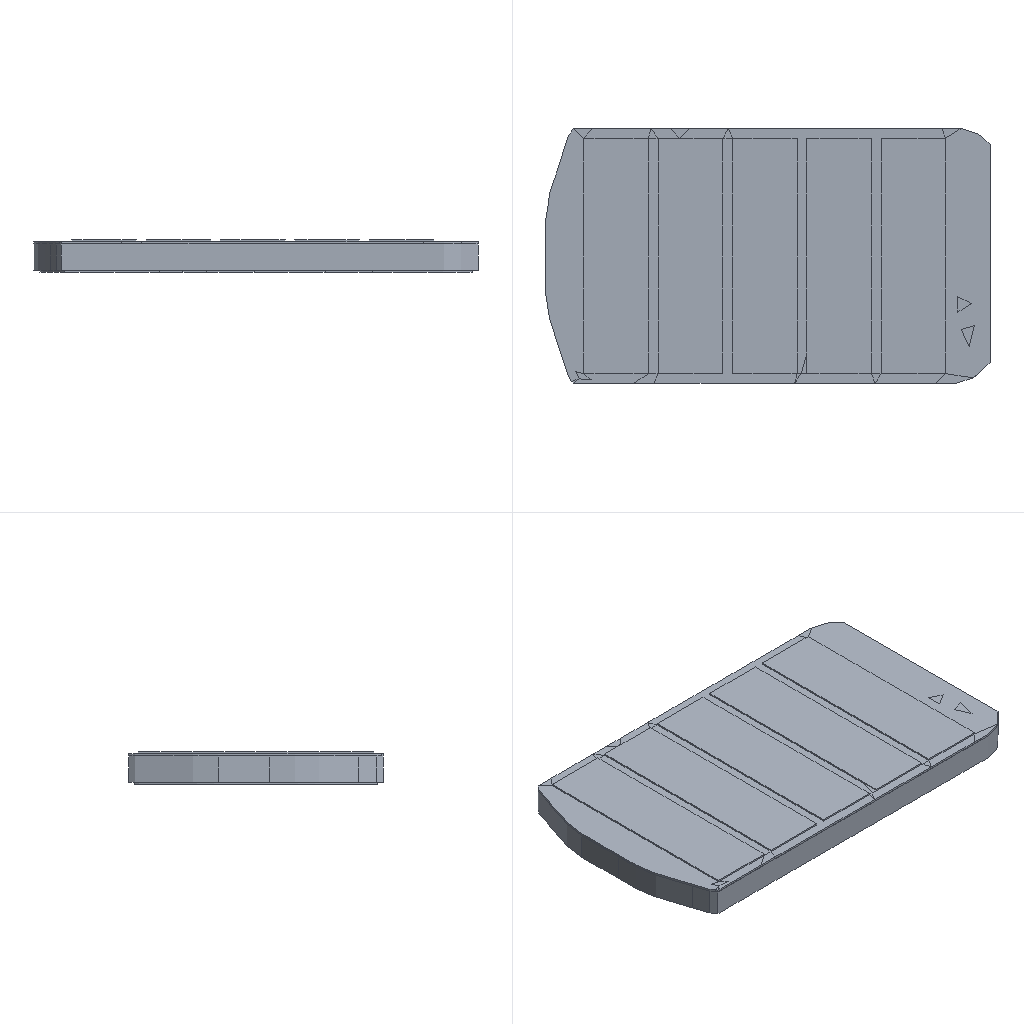Simulation study | abaqus
Set-up summary:
category,name,step,type,value,unit,region
solver,abaqus
solver,version,,,Abaqus/Standard 2020
units,not stated in the deck,,not stated
analysis,deck,,static,static
load_step,Step-2,Step-2,static,nlgeom=False
contact,interactions,,,general=1 pairs=0 ties=18
load_step,requested,,,1
mesh,nodes,,,72254
mesh,elements,,,47466
element_type,C3D6,,solid,272
element_type,SC6R,,solid_shell,576
element_type,SC8R,,solid_shell,17734
element_type,C3D8E,,solid,492
element_type,C3D8R,,solid,28392
load,load commands in deck,,count,1
bc,support commands in deck,,count,1
material,HT3_5222,,in results
material,PAOMO,,in results
material,Q235,,in results
material,YADIAN,,in results
check,setup vs results,,match,"per instance, exact: element labels, types and connectivity; labels of the nodes the elements use; coordinates of those nodes at SINGLE_PRECISION in 2 of 5 instance(s)"
Abaqus input file, long lists of numbers shortened:
*Heading
** Job name: Job-1 Model name: MODE_HT3
** Generated by: Abaqus/CAE 2020
*Preprint, echo=NO, model=NO, history=NO, contact=NO
**
** PARTS
**
*Part, name=battery
*Node
      1,         355.,          86.,         161.
      2,         355.,           0.,         161.
** (39652 more lines like these left out)
*Element, type=C3D6
 1,  5243,  5183,  5214, 20145, 20085, 20116
 2,  5231,  5232,  5254, 20133, 20134, 20156
** (270 more lines like these left out)
*Element, type=C3D8R
 17,  5183,   561,     1,     8, 20085,  5481,   640,   626
 18,   566,  5196,  5195,   567,  5353, 20098, 20097,  5352
** (28390 more lines like these left out)
*Nset, nset=Set-1, generate
     1,  39654,      1
*Elset, elset=Set-1, generate
     1,  28664,      1
*Nset, nset=Set-36, generate
     1,  39654,      1
*Elset, elset=Set-36, generate
     1,  28664,      1
** Section: Section-2
*Solid Section, elset=Set-1, material=paomo
,
*End Part
**
*Part, name=beam
*Node
      1,       1873.5,           8.,   7.5
      2,       1873.5,           0.,   7.5
** (11406 more lines like these left out)
*Element, type=SC8R
  1,   98,   93,    2,    1, 3561, 3203,  339,  459
  2,   97,   94,   93,   98, 3562, 3202, 3203, 3561
** (5232 more lines like these left out)
*Nset, nset=Set-5, generate
     1,  11408,      1
*Elset, elset=Set-5, generate
    1,  5234,     1
*Nset, nset=Set-82, generate
     1,  11408,      1
*Elset, elset=Set-82, generate
    1,  5234,     1
*Nset, nset=_PickedSet170, internal, generate
     1,  11408,      1
*Elset, elset=_PickedSet170, internal, generate
    1,  5234,     1
** Section: Section-1
*Shell Section, elset=_PickedSet170, material=Q235
2., 5
*End Part
**
*Part, name=shanggai
*Node
      1,   3817.754,  -593.33,         253.
      2,   3817.754,   593.33,         253.
** (1145 more lines like these left out)
*Element, type=SC8R
 1, 155, 625, 130,   1, 167, 647, 166,   6
 2, 625, 626, 131, 130, 647, 648, 165, 166
** (468 more lines like these left out)
*Element, type=SC6R
181,   23,   31,  405,  125,  118,  962
182,   52,  869,   53,  953, 1132,   99
** (32 more lines like these left out)
*Nset, nset=Set-4, generate
    1,  1147,     1
*Elset, elset=Set-4, generate
   1,  504,    1
*Nset, nset=_PickedSet401, internal, generate
    1,  1147,     1
*Elset, elset=_PickedSet401, internal, generate
   1,  504,    1
** Section: Section-1
*Shell Section, elset=_PickedSet401, material=Q235
2., 5
*End Part
**
*Part, name=xiangti
*Node
      1,        3160.,   537.25,         105.
      2,        3140.,   537.25,         105.
** (18731 more lines like these left out)
*Element, type=SC6R
  1,  1870,  1674,  1536,  7883,  7687,  7549
  2,   960,   717,   932,  6973,  6730,  6945
** (540 more lines like these left out)
*Element, type=SC8R
 266,  1016,   655,  5542,  1137,  7029,  6668, 11555,  7150
 267,   634,   661,   744,   831,  6647,  6674,  6757,  6844
** (12028 more lines like these left out)
*Nset, nset=Set-4
     1,     2,     3,     4,     5,     6,     7,     8,     9,    10,    11,    12,    13,    14,    15,    16
    17,    18,    19,    20,    21,    22,    23,    24,    25,    26,    27,    28,    29,    30,    31,    32
** (1150 more lines like these left out)
*Elset, elset=Set-4, generate
     1,  12444,      1
*Nset, nset=Set-5
    69,    70,    71,    72,    73,    74,    75,    76,    77,    78,    79,    80,    81,    82,    83,    84
   109,   110,   111,   112,   113,   114,   115,   116,   117,   118,   119,   120,   121,   122,   123,   124
** (21 more lines like these left out)
*Elset, elset=Set-5, generate
 12445,  12572,      1
*Nset, nset=_PickedSet106, internal, generate
     1,  18733,      1
*Elset, elset=_PickedSet106, internal, generate
     1,  12572,      1
** Section: Section-1
*Shell Section, elset=_PickedSet106, material=Q235
2., 5
*End Part
**
*Part, name=yadian
*Node
      1,  -998.167,   586.46,           0.
      2,  -910.396,   614.629,           0.
** (1310 more lines like these left out)
*Element, type=C3D8E
  1,  319,  121,   13,  142,  647,  449,  341,  470
  2,  121,  320,  141,   13,  449,  648,  469,  341
** (490 more lines like these left out)
*Nset, nset=Set-1, generate
    1,  1312,     1
*Elset, elset=Set-1, generate
   1,  492,    1
*Orientation, name=Ori-1
1., 0., 0., 0., 1., 0.
1, 0.
** Section: yadian
*Solid Section, elset=Set-1, orientation=Ori-1, material=yadian
,
*End Part
**
**
** ASSEMBLY
**
*Assembly, name=Assembly
**
*Instance, name=battery-1, part=battery
      2362.5,   558.832,         133.
      2362.5,   558.832,         133., 2363.5,   558.832,         133., 90.
*End Instance
**
*Instance, name=beam-1, part=beam
      2352.5,   612.334,         125.
      2352.5,   612.334,         125., 2353.5,   612.334,         125., 90.
*End Instance
**
*Instance, name=xiangti-1, part=xiangti
          0.,           0.,          15.
*End Instance
**
*Instance, name=shanggai-1, part=shanggai
          0.,           0., 26.
*End Instance
**
*Instance, name=yadian-1, part=yadian
 3331.429,     7.297,         125.
 3331.429,     7.297,         125.,  3331.429,     7.297,         126.,         180.
*End Instance
**
*Nset, nset=Set-20, instance=beam-1
   79,   80,   87,   89,   90, 2795, 2796, 2797, 2798, 2799, 2800, 2801, 2802, 2803, 2804, 2805
 2937, 2938, 2939, 2940, 2941, 2942, 2943, 2944, 2945, 2946, 2947, 2948
*Elset, elset=Set-20, instance=beam-1
 3662, 3783, 3784, 3785, 3786, 3787, 3788, 3789, 3790, 3791, 3792, 3793, 3794
*Nset, nset=Set-25, instance=beam-1
    2,    3,    5,    8,   93,   94,   95,  219,  220,  221,  222,  223,  224,  225,  226,  227
  228,  229,  230,  231,  232,  233,  234,  235,  236,  237,  238,  239,  240,  241,  242,  243
** (37 more lines like these left out)
*Elset, elset=Set-25, instance=beam-1, generate
   1,  484,    1
*Nset, nset=Set-35, instance=battery-1, generate
     1,  39654,      1
*Elset, elset=Set-35, instance=battery-1, generate
     1,  28664,      1
*Nset, nset=Set-36, instance=xiangti-1
   1,   2,   3,   4,   5,   6,   7,   8,   9,  10,  11,  12,  13,  14,  15,  16
  17,  18,  19,  20,  21,  22,  23,  24,  85,  86,  87,  88,  89,  90,  91,  92
** (7 more lines like these left out)
*Elset, elset=Set-36, instance=xiangti-1
  6226,  6230,  6232,  6234,  6236,  6237,  6238,  6239,  6251,  6253,  6255,  6263,  6269,  6272,  6274,  6277
  6279,  6284,  6286,  6295,  6302,  6307,  6309,  6311,  6323,  6326,  6332,  6334,  6340,  6343,  6352,  6356
** (3 more lines like these left out)
*Nset, nset=Set-37, instance=battery-1, generate
     1,  39654,      1
*Nset, nset=Set-37, instance=beam-1, generate
     1,  11408,      1
*Nset, nset=Set-37, instance=xiangti-1, generate
     1,  18733,      1
*Nset, nset=Set-37, instance=yadian-1, generate
    1,  1312,     1
*Nset, nset=Set-37, instance=shanggai-1, generate
    1,  1147,     1
*Elset, elset=Set-37, instance=battery-1, generate
     1,  28664,      1
*Elset, elset=Set-37, instance=beam-1, generate
    1,  5234,     1
*Elset, elset=Set-37, instance=xiangti-1, generate
     1,  12572,      1
*Elset, elset=Set-37, instance=yadian-1, generate
   1,  492,    1
*Elset, elset=Set-37, instance=shanggai-1, generate
   1,  504,    1
*Nset, nset=Set-38, instance=yadian-1, generate
    1,  1312,     1
*Elset, elset=Set-38, instance=yadian-1, generate
   1,  492,    1
*Elset, elset=_BATTERY_S6, internal, instance=battery-1
    18,    25,    26,    29,    32,    33,    57,    61,    68,   118,   125,   126,   129,   132,   133,   157
   161,   168,   218,   225,   226,   229,   232,   233,   257,   261,   268,   318,   325,   326,   329,   332
** (178 more lines like these left out)
*Elset, elset=_BATTERY_S4, internal, instance=battery-1
    23,    30,    34,    35,    36,    55,    56,    71,   123,   130,   134,   135,   136,   155,   156,   171
   223,   230,   234,   235,   236,   255,   256,   271,   323,   330,   334,   335,   336,   355,   356,   371
** (115 more lines like these left out)
*Elset, elset=_BATTERY_S3, internal, instance=battery-1
    37,   137,   237,   337,   437,   537,   637,   737,   820,   841,   922,   943,  1024,  1045,  1126,  1147
  1228,  1249,  1330,  1351,  1432,  1453,  1534,  1555,  1657,  1759,  1861,  1963,  2065,  2167,  2269,  2371
** (17 more lines like these left out)
*Surface, type=ELEMENT, name=BATTERY
_BATTERY_S6, S6
_BATTERY_S4, S4
_BATTERY_S3, S3
*Elset, elset=_BATTERY1_S6, internal, instance=battery-1
    18,    25,    26,    29,    32,    33,    57,    61,    68,   118,   125,   126,   129,   132,   133,   157
   161,   168,   218,   225,   226,   229,   232,   233,   257,   261,   268,   318,   325,   326,   329,   332
** (33 more lines like these left out)
*Elset, elset=_BATTERY1_S4, internal, instance=battery-1
    23,    30,    34,    35,    36,    55,    56,    71,   123,   130,   134,   135,   136,   155,   156,   171
   223,   230,   234,   235,   236,   255,   256,   271,   323,   330,   334,   335,   336,   355,   356,   371
** (23 more lines like these left out)
*Elset, elset=_BATTERY1_S3, internal, instance=battery-1
    37,   137,   237,   337,   437,   537,   637,   737,  1657,  1759,  1861,  1963,  2065,  2167,  2269,  2371
 13116, 13216, 13316, 13416, 13516, 13616, 13716, 13816, 14768, 14871, 14974, 15077, 15180, 15283, 15386, 15489
** (2 more lines like these left out)
*Surface, type=ELEMENT, name=BATTERY1
_BATTERY1_S6, S6
_BATTERY1_S4, S4
_BATTERY1_S3, S3
*Elset, elset=_BATTERY2_S4, internal, instance=battery-1
  4083,  4084,  4089,  4090,  4114,  4122,  4123,  4125,  4127,  4128,  4129,  4185,  4186,  4191,  4192,  4216
  4224,  4225,  4227,  4229,  4230,  4231,  4287,  4288,  4293,  4294,  4318,  4326,  4327,  4329,  4331,  4332
** (22 more lines like these left out)
*Elset, elset=_BATTERY2_S6, internal, instance=battery-1
  4099,  4104,  4109,  4112,  4117,  4131,  4201,  4206,  4211,  4214,  4219,  4233,  4303,  4308,  4313,  4316
  4321,  4335,  4405,  4410,  4415,  4418,  4423,  4437,  4507,  4512,  4517,  4520,  4525,  4539,  4609,  4614
** (34 more lines like these left out)
*Elset, elset=_BATTERY2_S3, internal, instance=battery-1
  4105,  4207,  4309,  4411,  4513,  4615,  4717,  4819,  4934,  5034,  5134,  5234,  5334,  5434,  5534,  5634
  8198,  8298,  8398,  8498,  8598,  8698,  8798,  8898, 11495, 11598, 11701, 11804, 11907, 12010, 12113, 12216
** (2 more lines like these left out)
*Surface, type=ELEMENT, name=BATTERY2
_BATTERY2_S4, S4
_BATTERY2_S6, S6
_BATTERY2_S3, S3
*Elset, elset=_BATTERY3_S4, internal, instance=battery-1
  2451,  2452,  2453,  2457,  2458,  2462,  2482,  2490,  2491,  2493,  2495,  2499,  2553,  2554,  2555,  2559
  2560,  2564,  2584,  2592,  2593,  2595,  2597,  2601,  2655,  2656,  2657,  2661,  2662,  2666,  2686,  2694
** (22 more lines like these left out)
*Elset, elset=_BATTERY3_S6, internal, instance=battery-1
  2467,  2472,  2478,  2485,  2497,  2569,  2574,  2580,  2587,  2599,  2671,  2676,  2682,  2689,  2701,  2773
  2778,  2784,  2791,  2803,  2875,  2880,  2886,  2893,  2905,  2977,  2982,  2988,  2995,  3007,  3079,  3084
** (34 more lines like these left out)
*Elset, elset=_BATTERY3_S3, internal, instance=battery-1
  2473,  2575,  2677,  2779,  2881,  2983,  3085,  3187,  7381,  7481,  7581,  7681,  7781,  7881,  7981,  8081
  9013,  9113,  9213,  9313,  9413,  9513,  9613,  9713, 10671, 10774, 10877, 10980, 11083, 11186, 11289, 11392
** (2 more lines like these left out)
*Surface, type=ELEMENT, name=BATTERY3
_BATTERY3_S4, S4
_BATTERY3_S6, S6
_BATTERY3_S3, S3
*Elset, elset=_BATTERY4_S4, internal, instance=battery-1
  3265,  3267,  3273,  3300,  3305,  3306,  3307,  3308,  3309,  3367,  3369,  3375,  3402,  3407,  3408,  3409
  3410,  3411,  3469,  3471,  3477,  3504,  3509,  3510,  3511,  3512,  3513,  3571,  3573,  3579,  3606,  3611
** (20 more lines like these left out)
*Elset, elset=_BATTERY4_S3, internal, instance=battery-1
  3268,  3289,  3370,  3391,  3472,  3493,  3574,  3595,  3676,  3697,  3778,  3799,  3880,  3901,  3982,  4003
  5749,  5849,  5949,  6049,  6149,  6249,  6349,  6449,  6566,  6666,  6766,  6866,  6966,  7066,  7166,  7266
** (2 more lines like these left out)
*Elset, elset=_BATTERY4_S6, internal, instance=battery-1
  3283,  3288,  3293,  3296,  3299,  3301,  3311,  3385,  3390,  3395,  3398,  3401,  3403,  3413,  3487,  3492
  3497,  3500,  3503,  3505,  3515,  3589,  3594,  3599,  3602,  3605,  3607,  3617,  3691,  3696,  3701,  3704
** (36 more lines like these left out)
*Surface, type=ELEMENT, name=BATTERY4
_BATTERY4_S4, S4
_BATTERY4_S3, S3
_BATTERY4_S6, S6
*Elset, elset=_BATTERY5_S4, internal, instance=battery-1
   819,   825,   830,   842,   849,   857,   858,   860,   921,   927,   932,   944,   951,   959,   960,   962
  1023,  1029,  1034,  1046,  1053,  1061,  1062,  1064,  1125,  1131,  1136,  1148,  1155,  1163,  1164,  1166
** (22 more lines like these left out)
*Elset, elset=_BATTERY5_S3, internal, instance=battery-1
   820,   841,   922,   943,  1024,  1045,  1126,  1147,  1228,  1249,  1330,  1351,  1432,  1453,  1534,  1555
 18853, 18953, 19053, 19153, 19253, 19353, 19453, 19553, 20513, 20616, 20719, 20822, 20925, 21028, 21131, 21234
** (2 more lines like these left out)
*Elset, elset=_BATTERY5_S6, internal, instance=battery-1
   827,   835,   840,   845,   847,   852,   866,   868,   929,   937,   942,   947,   949,   954,   968,   970
  1031,  1039,  1044,  1049,  1051,  1056,  1070,  1072,  1133,  1141,  1146,  1151,  1153,  1158,  1172,  1174
** (33 more lines like these left out)
*Surface, type=ELEMENT, name=BATTERY5
_BATTERY5_S4, S4
_BATTERY5_S3, S3
_BATTERY5_S6, S6
*Elset, elset=_BEAM_S6, internal, instance=beam-1
    1,    2,    3,    4,    5,    6,    7,    8,    9,   10,   11,   12,   13,   14,   15,   16
   17,   18,   19,   20,   21,   22,   23,   24,   25,   26,   27,   28,   29,   30,   31,   32
** (59 more lines like these left out)
*Elset, elset=_BEAM_S1, internal, instance=beam-1
 2218, 2219, 2220, 2221, 2222, 2223, 2224, 2225, 2226, 2227, 2228, 2229, 2230, 2231, 2232, 2233
 2234, 2235, 2236, 2237, 2238, 2239, 2240, 2241, 2242, 2243, 2244, 2245, 2246, 2247, 2248, 2249
** (18 more lines like these left out)
*Surface, type=ELEMENT, name=BEAM
_BEAM_S6, S6
_BEAM_S1, S1
*Elset, elset=_DIMIANCE_S2, internal, instance=xiangti-1, generate
  6223,  12444,      1
*Surface, type=ELEMENT, name=DIMIANCE
_DIMIANCE_S2, S2
*Elset, elset=_FUABN9_S1, internal, instance=beam-1, generate
 3138,  3177,     1
*Surface, type=ELEMENT, name=FUABN9
_FUABN9_S1, S1
*Elset, elset=_FUBAN1_S6, internal, instance=beam-1, generate
 3178,  3661,     1
*Surface, type=ELEMENT, name=FUBAN1
_FUBAN1_S6, S6
*Elset, elset=_FUBAN2_S1, internal, instance=beam-1, generate
 2218,  2257,     1
*Surface, type=ELEMENT, name=FUBAN2
_FUBAN2_S1, S1
*Elset, elset=_FUBAN3_S1, internal, instance=beam-1, generate
 2298,  2337,     1
*Surface, type=ELEMENT, name=FUBAN3
_FUBAN3_S1, S1
*Elset, elset=_FUBAN4_S1, internal, instance=beam-1, generate
 2498,  2537,     1
*Surface, type=ELEMENT, name=FUBAN4
_FUBAN4_S1, S1
*Elset, elset=_FUBAN5_S1, internal, instance=beam-1, generate
 2578,  2617,     1
*Surface, type=ELEMENT, name=FUBAN5
_FUBAN5_S1, S1
*Elset, elset=_FUBAN6_S1, internal, instance=beam-1, generate
 2778,  2817,     1
*Surface, type=ELEMENT, name=FUBAN6
_FUBAN6_S1, S1
*Elset, elset=_FUBAN7_S1, internal, instance=beam-1, generate
 2858,  2897,     1
*Surface, type=ELEMENT, name=FUBAN7
_FUBAN7_S1, S1
*Elset, elset=_FUBAN8_S1, internal, instance=beam-1, generate
 3058,  3097,     1
*Surface, type=ELEMENT, name=FUBAN8
_FUBAN8_S1, S1
*Elset, elset=_FUBAN10_S6, internal, instance=beam-1, generate
   1,  484,    1
*Surface, type=ELEMENT, name=FUBAN10
_FUBAN10_S6, S6
*Elset, elset=_b1_S4, internal, instance=beam-1, generate
 3178,  3661,     1
*Surface, type=ELEMENT, name=b1
_b1_S4, S4
*Elset, elset=_b2_S2, internal, instance=beam-1, generate
 2218,  2337,     1
*Surface, type=ELEMENT, name=b2
_b2_S2, S2
*Elset, elset=_b3_S2, internal, instance=beam-1, generate
 2498,  2617,     1
*Surface, type=ELEMENT, name=b3
_b3_S2, S2
*Elset, elset=_b4_S2, internal, instance=beam-1, generate
 2778,  2897,     1
*Surface, type=ELEMENT, name=b4
_b4_S2, S2
*Elset, elset=_b5_S2, internal, instance=beam-1, generate
 3058,  3177,     1
*Surface, type=ELEMENT, name=b5
_b5_S2, S2
*Elset, elset=_b6_S4, internal, instance=beam-1, generate
   1,  484,    1
*Surface, type=ELEMENT, name=b6
_b6_S4, S4
*Elset, elset=_beam1_S6, internal, instance=beam-1
  485, 2258, 2577, 2857, 3098
*Elset, elset=_beam1_S3, internal, instance=beam-1
 2046, 2047, 2048, 2049, 2050, 2051, 2052, 2053, 2054, 2055, 2056, 2057, 2214, 2215, 2216, 2217
 2257, 2337, 2494, 2495, 2496, 2497, 2537, 2617, 2774, 2775, 2776, 2777, 2817, 2897, 3054, 3055
** (1 more lines like these left out)
*Elset, elset=_beam1_S1, internal, instance=beam-1, generate
 1,  4,  1
*Elset, elset=_beam1_S2, internal, instance=beam-1, generate
 3658,  3661,     1
*Elset, elset=_beam1_S4, internal, instance=beam-1
 3782,
*Surface, type=ELEMENT, name=beam1
_beam1_S6, S6
_beam1_S3, S3
_beam1_S2, S2
_beam1_S4, S4
_beam1_S1, S1
*Elset, elset=_beam2_S1, internal, instance=beam-1, generate
 1,  4,  1
*Elset, elset=_beam2_S4, internal, instance=beam-1
  605, 2297, 2538, 2818, 3137
*Elset, elset=_beam2_S5, internal, instance=beam-1
  606,  607,  608,  609,  610,  611,  612,  613,  614,  615,  616,  617, 2058, 2059, 2060, 2061
 2218, 2298, 2338, 2339, 2340, 2341, 2498, 2578, 2618, 2619, 2620, 2621, 2778, 2858, 2898, 2899
** (1 more lines like these left out)
*Elset, elset=_beam2_S2, internal, instance=beam-1, generate
 3658,  3661,     1
*Elset, elset=_beam2_S6, internal, instance=beam-1
 3662,
*Surface, type=ELEMENT, name=beam2
_beam2_S1, S1
_beam2_S4, S4
_beam2_S2, S2
_beam2_S6, S6
_beam2_S5, S5
*Elset, elset=_ceban1_S5, internal, instance=xiangti-1
 12475, 12499, 12502, 12533, 12557, 12560
*Elset, elset=_ceban1_S6, internal, instance=xiangti-1
 12478, 12504, 12536, 12562
*Elset, elset=_ceban1_S3, internal, instance=xiangti-1
 12495, 12496, 12497, 12498, 12500, 12501, 12512, 12553, 12554, 12555, 12556, 12558, 12559, 12570
*Elset, elset=_ceban1_S4, internal, instance=xiangti-1
 12503, 12505, 12513, 12514, 12561, 12563, 12571, 12572
*Surface, type=ELEMENT, name=ceban1
_ceban1_S5, S5
_ceban1_S6, S6
_ceban1_S4, S4
_ceban1_S3, S3
*Elset, elset=_ceban2_S6, internal, instance=xiangti-1
 12462, 12520
*Elset, elset=_ceban2_S5, internal, instance=xiangti-1
 12463, 12488, 12491, 12493, 12521, 12546, 12549, 12551
*Elset, elset=_ceban2_S3, internal, instance=xiangti-1
 12484, 12485, 12486, 12487, 12489, 12490, 12492, 12494, 12507, 12508, 12509, 12542, 12543, 12544, 12545, 12547
 12548, 12550, 12552, 12565, 12566, 12567
*Surface, type=ELEMENT, name=ceban2
_ceban2_S6, S6
_ceban2_S5, S5
_ceban2_S3, S3
*Elset, elset=_cebanshang_S2, internal, instance=xiangti-1
 12451, 12452, 12453, 12454, 12455, 12456, 12515, 12516, 12517, 12518, 12519, 12520, 12521, 12522, 12523, 12524
 12525, 12526, 12527, 12528, 12529, 12530, 12531, 12532, 12533, 12534, 12535, 12536, 12537, 12538, 12539, 12540
** (2 more lines like these left out)
*Surface, type=ELEMENT, name=cebanshang
_cebanshang_S2, S2
*Elset, elset=_fuban_S4, internal, instance=beam-1
    1,    2,    3,    4,    5,    6,    7,    8,    9,   10,   11,   12,   13,   14,   15,   16
   17,   18,   19,   20,   21,   22,   23,   24,   25,   26,   27,   28,   29,   30,   31,   32
** (59 more lines like these left out)
*Elset, elset=_fuban_S2, internal, instance=beam-1
 2218, 2219, 2220, 2221, 2222, 2223, 2224, 2225, 2226, 2227, 2228, 2229, 2230, 2231, 2232, 2233
 2234, 2235, 2236, 2237, 2238, 2239, 2240, 2241, 2242, 2243, 2244, 2245, 2246, 2247, 2248, 2249
** (28 more lines like these left out)
*Surface, type=ELEMENT, name=fuban
_fuban_S4, S4
_fuban_S2, S2
*Elset, elset=_m_Surf-37_S6, internal, instance=xiangti-1
 12458, 12460, 12462, 12467, 12470, 12477, 12478, 12482, 12504, 12516, 12518, 12520, 12525, 12528, 12535, 12536
 12540, 12562
*Elset, elset=_m_Surf-37_S5, internal, instance=xiangti-1
 12446, 12447, 12452, 12453, 12461, 12463, 12471, 12473, 12475, 12488, 12491, 12493, 12499, 12502, 12506, 12519
 12521, 12529, 12531, 12533, 12546, 12549, 12551, 12557, 12560, 12564
*Elset, elset=_m_Surf-37_S3, internal, instance=xiangti-1
 12457, 12468, 12469, 12472, 12474, 12476, 12479, 12484, 12485, 12486, 12487, 12489, 12490, 12492, 12494, 12495
 12496, 12497, 12498, 12500, 12501, 12507, 12508, 12509, 12512, 12515, 12526, 12527, 12530, 12532, 12534, 12537
** (2 more lines like these left out)
*Elset, elset=_m_Surf-37_S4, internal, instance=xiangti-1
 12449, 12455, 12459, 12466, 12480, 12481, 12483, 12503, 12505, 12510, 12511, 12513, 12514, 12517, 12524, 12538
 12539, 12541, 12561, 12563, 12568, 12569, 12571, 12572
*Surface, type=ELEMENT, name=m_Surf-37
_m_Surf-37_S6, S6
_m_Surf-37_S5, S5
_m_Surf-37_S4, S4
_m_Surf-37_S3, S3
*Elset, elset=_s_Surf-37_S6, internal, instance=yadian-1
   3,   4,   6,   7,   8,   9,  10,  11,  12,  14,  35,  36,  37,  38,  39,  40
  42,  48,  49,  50,  51,  53,  54,  55,  56,  61,  81, 100, 101, 105, 118, 119
** (6 more lines like these left out)
*Elset, elset=_s_Surf-37_S3, internal, instance=yadian-1
   1,   2,  13,  15,  16,  19,  21,  23,  24,  25,  26,  27,  28,  29,  30,  43
  44,  46,  58,  59,  62,  64,  83,  84,  85,  86,  87,  88,  89,  90,  91,  92
** (15 more lines like these left out)
*Elset, elset=_s_Surf-37_S5, internal, instance=yadian-1
  17,  18,  20,  22,  31,  32,  33,  34,  41,  45,  47,  57,  60,  63,  65,  66
  67,  68,  69,  70,  71,  72,  73,  74,  75,  76,  77,  78,  79,  80,  82, 181
** (4 more lines like these left out)
*Elset, elset=_s_Surf-37_S4, internal, instance=yadian-1
   5,  52, 146, 169, 216, 310, 333, 380, 474
*Surface, type=ELEMENT, name=s_Surf-37
_s_Surf-37_S6, S6
_s_Surf-37_S3, S3
_s_Surf-37_S4, S4
_s_Surf-37_S5, S5
*Elset, elset=_shanggai_S2, internal, instance=shanggai-1
 198, 199, 200, 201, 202, 203, 204, 205, 206, 207, 208, 209, 210, 211, 212, 213
 214, 360, 361, 362, 363, 364, 365, 366, 367, 368, 369, 370, 371, 372, 373, 374
** (9 more lines like these left out)
*Surface, type=ELEMENT, name=shanggai
_shanggai_S2, S2
** Constraint: Constraint-1
*Tie, name=Constraint-1, adjust=yes, type=SURFACE TO SURFACE
shanggai, cebanshang
** Constraint: Constraint-8
*Tie, name=Constraint-8, adjust=yes
BATTERY1, FUBAN1
** Constraint: Constraint-9
*Tie, name=Constraint-9, adjust=yes
BATTERY1, FUBAN2
** Constraint: Constraint-10
*Tie, name=Constraint-10, adjust=yes
BATTERY2, FUBAN3
** Constraint: Constraint-11
*Tie, name=Constraint-11, adjust=yes
BATTERY2, FUBAN4
** Constraint: Constraint-12
*Tie, name=Constraint-12, adjust=yes
BATTERY3, FUBAN5
** Constraint: Constraint-13
*Tie, name=Constraint-13, adjust=yes, type=SURFACE TO SURFACE
b1, DIMIANCE
** Constraint: Constraint-14
*Tie, name=Constraint-14, adjust=yes, type=SURFACE TO SURFACE
b2, DIMIANCE
** Constraint: Constraint-15
*Tie, name=Constraint-15, adjust=yes, type=SURFACE TO SURFACE
b4, DIMIANCE
** Constraint: Constraint-16
*Tie, name=Constraint-16, adjust=yes, type=SURFACE TO SURFACE
b3, DIMIANCE
** Constraint: Constraint-17
*Tie, name=Constraint-17, adjust=yes, type=SURFACE TO SURFACE
b5, DIMIANCE
** Constraint: Constraint-18
*Tie, name=Constraint-18, adjust=yes, type=SURFACE TO SURFACE
b6, DIMIANCE
** Constraint: Constraint-19
*Tie, name=Constraint-19, adjust=yes
BATTERY3, FUBAN6
** Constraint: Constraint-20
*Tie, name=Constraint-20, adjust=yes
BATTERY4, FUBAN7
** Constraint: Constraint-21
*Tie, name=Constraint-21, adjust=yes
BATTERY4, FUBAN8
** Constraint: Constraint-22
*Tie, name=Constraint-22, adjust=yes
BATTERY5, FUABN9
** Constraint: Constraint-23
*Tie, name=Constraint-23, adjust=yes
BATTERY5, FUBAN10
** Constraint: yadian
*Tie, name=yadian, adjust=yes
s_Surf-37, m_Surf-37
*Elset, elset=__Int-1_gcs0_444_S3, internal, instance=xiangti-1
 275, 350
*Elset, elset=__Int-1_gcs0_444_S6, internal, instance=xiangti-1
 279, 280
*Elset, elset=__Int-1_gcs0_444_S5, internal, instance=xiangti-1
 294,
*Elset, elset=__Int-1_gcs0_444_S4, internal, instance=xiangti-1
 375,
*Surface, type=ELEMENT, name=_Int-1_gcs0_444, internal
__Int-1_gcs0_444_S3, S3
__Int-1_gcs0_444_S6, S6
__Int-1_gcs0_444_S4, S4
__Int-1_gcs0_444_S5, S5
*Elset, elset=__Int-1_gcs0_445_S4, internal, instance=xiangti-1
 298, 399, 425, 432, 570
*Elset, elset=__Int-1_gcs0_445_S3, internal, instance=xiangti-1
 429,
*Surface, type=ELEMENT, name=_Int-1_gcs0_445, internal
__Int-1_gcs0_445_S4, S4
__Int-1_gcs0_445_S3, S3
*Elset, elset=__Int-1_gcs0_446_S5, internal, instance=xiangti-1
 281,
*Elset, elset=__Int-1_gcs0_446_S4, internal, instance=xiangti-1
 383, 410, 437, 470
*Elset, elset=__Int-1_gcs0_446_S6, internal, instance=xiangti-1
 548,
*Surface, type=ELEMENT, name=_Int-1_gcs0_446, internal
__Int-1_gcs0_446_S5, S5
__Int-1_gcs0_446_S4, S4
__Int-1_gcs0_446_S6, S6
*Elset, elset=__Int-1_gcs0_447_S3, internal, instance=xiangti-1
 317,
*Elset, elset=__Int-1_gcs0_447_S4, internal, instance=xiangti-1
 404, 413, 433, 481
*Elset, elset=__Int-1_gcs0_447_S5, internal, instance=xiangti-1
 405,
*Surface, type=ELEMENT, name=_Int-1_gcs0_447, internal
__Int-1_gcs0_447_S3, S3
__Int-1_gcs0_447_S4, S4
__Int-1_gcs0_447_S5, S5
*Elset, elset=__Int-1_gcs0_448_S4, internal, instance=xiangti-1
 306, 352, 377, 423
*Elset, elset=__Int-1_gcs0_448_S3, internal, instance=xiangti-1
 338,
*Elset, elset=__Int-1_gcs0_448_S6, internal, instance=xiangti-1
 475,
*Surface, type=ELEMENT, name=_Int-1_gcs0_448, internal
__Int-1_gcs0_448_S4, S4
__Int-1_gcs0_448_S3, S3
__Int-1_gcs0_448_S6, S6
*Elset, elset=__Int-1_gcs0_449_S4, internal, instance=xiangti-1
   4, 312, 320
*Elset, elset=__Int-1_gcs0_449_S6, internal, instance=xiangti-1
 315, 345, 416
*Surface, type=ELEMENT, name=_Int-1_gcs0_449, internal
__Int-1_gcs0_449_S4, S4
__Int-1_gcs0_449_S6, S6
*Elset, elset=__Int-1_gcs0_450_S5, internal, instance=xiangti-1
 322,
*Elset, elset=__Int-1_gcs0_450_S4, internal, instance=xiangti-1
 386, 438, 574
*Elset, elset=__Int-1_gcs0_450_S3, internal, instance=xiangti-1
 442, 461
*Surface, type=ELEMENT, name=_Int-1_gcs0_450, internal
__Int-1_gcs0_450_S5, S5
__Int-1_gcs0_450_S4, S4
__Int-1_gcs0_450_S3, S3
*Elset, elset=__Int-1_gcs0_451_S4, internal, instance=xiangti-1
   7, 329, 354, 445
*Elset, elset=__Int-1_gcs0_451_S3, internal, instance=xiangti-1
 504, 516
*Surface, type=ELEMENT, name=_Int-1_gcs0_451, internal
__Int-1_gcs0_451_S4, S4
__Int-1_gcs0_451_S3, S3
*Elset, elset=__Int-1_gcs0_452_S5, internal, instance=xiangti-1
 327,
*Elset, elset=__Int-1_gcs0_452_S4, internal, instance=xiangti-1
 395, 420
*Elset, elset=__Int-1_gcs0_452_S6, internal, instance=xiangti-1
 418, 458
*Elset, elset=__Int-1_gcs0_452_S3, internal, instance=xiangti-1
 550,
*Surface, type=ELEMENT, name=_Int-1_gcs0_452, internal
__Int-1_gcs0_452_S5, S5
__Int-1_gcs0_452_S4, S4
__Int-1_gcs0_452_S6, S6
__Int-1_gcs0_452_S3, S3
*Elset, elset=__Int-1_gcs0_453_S4, internal, instance=xiangti-1
 282, 366, 411, 451, 604
*Elset, elset=__Int-1_gcs0_453_S5, internal, instance=xiangti-1
 369,
*Surface, type=ELEMENT, name=_Int-1_gcs0_453, internal
__Int-1_gcs0_453_S4, S4
__Int-1_gcs0_453_S5, S5
*Elset, elset=__Int-1_gcs0_454_S3, internal, instance=xiangti-1
 296, 406, 483
*Elset, elset=__Int-1_gcs0_454_S4, internal, instance=xiangti-1
 407, 421
*Elset, elset=__Int-1_gcs0_454_S5, internal, instance=xiangti-1
 422,
*Surface, type=ELEMENT, name=_Int-1_gcs0_454, internal
__Int-1_gcs0_454_S3, S3
__Int-1_gcs0_454_S4, S4
__Int-1_gcs0_454_S5, S5
*Elset, elset=__Int-1_gcs0_455_S4, internal, instance=xiangti-1
 269,
*Elset, elset=__Int-1_gcs0_455_S5, internal, instance=xiangti-1
 273, 277, 408
*Elset, elset=__Int-1_gcs0_455_S3, internal, instance=xiangti-1
 491, 527
*Surface, type=ELEMENT, name=_Int-1_gcs0_455, internal
__Int-1_gcs0_455_S4, S4
__Int-1_gcs0_455_S5, S5
__Int-1_gcs0_455_S3, S3
*Elset, elset=__Int-1_gcs0_508_S5, internal, instance=xiangti-1
 6286, 6311, 6402
*Elset, elset=__Int-1_gcs0_508_S6, internal, instance=xiangti-1
 6461, 6473
*Elset, elset=__Int-1_gcs0_508_S4, internal, instance=xiangti-1
 12186,
*Surface, type=ELEMENT, name=_Int-1_gcs0_508, internal
__Int-1_gcs0_508_S5, S5
__Int-1_gcs0_508_S6, S6
__Int-1_gcs0_508_S4, S4
*Elset, elset=__Int-1_gcs0_509_S4, internal, instance=xiangti-1
 6284,
*Elset, elset=__Int-1_gcs0_509_S5, internal, instance=xiangti-1
 6352, 6377
*Elset, elset=__Int-1_gcs0_509_S3, internal, instance=xiangti-1
 6375, 6415
*Elset, elset=__Int-1_gcs0_509_S6, internal, instance=xiangti-1
 6507,
*Surface, type=ELEMENT, name=_Int-1_gcs0_509, internal
__Int-1_gcs0_509_S4, S4
__Int-1_gcs0_509_S5, S5
__Int-1_gcs0_509_S6, S6
__Int-1_gcs0_509_S3, S3
*Elset, elset=__Int-1_gcs0_510_S6, internal, instance=xiangti-1
 6253, 6363, 6440
*Elset, elset=__Int-1_gcs0_510_S5, internal, instance=xiangti-1
 6364, 6378
*Elset, elset=__Int-1_gcs0_510_S4, internal, instance=xiangti-1
 6379,
*Surface, type=ELEMENT, name=_Int-1_gcs0_510, internal
__Int-1_gcs0_510_S6, S6
__Int-1_gcs0_510_S5, S5
__Int-1_gcs0_510_S4, S4
*Elset, elset=__Int-1_gcs0_511_S5, internal, instance=xiangti-1
 6226,
*Elset, elset=__Int-1_gcs0_511_S4, internal, instance=xiangti-1
 6230, 6234, 6365
*Elset, elset=__Int-1_gcs0_511_S6, internal, instance=xiangti-1
 6448, 6484
*Surface, type=ELEMENT, name=_Int-1_gcs0_511, internal
__Int-1_gcs0_511_S5, S5
__Int-1_gcs0_511_S4, S4
__Int-1_gcs0_511_S6, S6
*Elset, elset=__Int-1_gcs0_512_S5, internal, instance=xiangti-1
 6263, 6309, 6334, 6380
*Elset, elset=__Int-1_gcs0_512_S6, internal, instance=xiangti-1
 6295,
*Elset, elset=__Int-1_gcs0_512_S3, internal, instance=xiangti-1
 6432,
*Surface, type=ELEMENT, name=_Int-1_gcs0_512, internal
__Int-1_gcs0_512_S5, S5
__Int-1_gcs0_512_S6, S6
__Int-1_gcs0_512_S3, S3
*Elset, elset=__Int-1_gcs0_513_S6, internal, instance=xiangti-1
 6274,
*Elset, elset=__Int-1_gcs0_513_S5, internal, instance=xiangti-1
 6361, 6370, 6390, 6438
*Elset, elset=__Int-1_gcs0_513_S4, internal, instance=xiangti-1
 6362,
*Surface, type=ELEMENT, name=_Int-1_gcs0_513, internal
__Int-1_gcs0_513_S6, S6
__Int-1_gcs0_513_S5, S5
__Int-1_gcs0_513_S4, S4
*Elset, elset=__Int-1_gcs0_514_S5, internal, instance=xiangti-1
 6255, 6356, 6382, 6389, 6527
*Elset, elset=__Int-1_gcs0_514_S6, internal, instance=xiangti-1
 6386,
*Surface, type=ELEMENT, name=_Int-1_gcs0_514, internal
__Int-1_gcs0_514_S5, S5
__Int-1_gcs0_514_S6, S6
*Elset, elset=__Int-1_gcs0_515_S6, internal, instance=xiangti-1
 6232, 6307
*Elset, elset=__Int-1_gcs0_515_S3, internal, instance=xiangti-1
 6236, 6237
*Elset, elset=__Int-1_gcs0_515_S4, internal, instance=xiangti-1
 6251,
*Elset, elset=__Int-1_gcs0_515_S5, internal, instance=xiangti-1
 6332,
*Surface, type=ELEMENT, name=_Int-1_gcs0_515, internal
__Int-1_gcs0_515_S6, S6
__Int-1_gcs0_515_S3, S3
__Int-1_gcs0_515_S4, S4
__Int-1_gcs0_515_S5, S5
*Elset, elset=__Int-1_gcs0_516_S5, internal, instance=xiangti-1
 6269, 6277
*Elset, elset=__Int-1_gcs0_516_S3, internal, instance=xiangti-1
 6272, 6302, 6373
*Elset, elset=__Int-1_gcs0_516_S4, internal, instance=xiangti-1
 12183,
*Surface, type=ELEMENT, name=_Int-1_gcs0_516, internal
__Int-1_gcs0_516_S5, S5
__Int-1_gcs0_516_S3, S3
__Int-1_gcs0_516_S4, S4
*Elset, elset=__Int-1_gcs0_517_S4, internal, instance=xiangti-1
 6279,
*Elset, elset=__Int-1_gcs0_517_S5, internal, instance=xiangti-1
 6343, 6395, 6531
*Elset, elset=__Int-1_gcs0_517_S6, internal, instance=xiangti-1
 6399, 6418
*Surface, type=ELEMENT, name=_Int-1_gcs0_517, internal
__Int-1_gcs0_517_S4, S4
__Int-1_gcs0_517_S5, S5
__Int-1_gcs0_517_S6, S6
*Elset, elset=__Int-1_gcs0_518_S4, internal, instance=xiangti-1
 6238,
*Elset, elset=__Int-1_gcs0_518_S5, internal, instance=xiangti-1
 6340, 6367, 6394, 6427
*Elset, elset=__Int-1_gcs0_518_S3, internal, instance=xiangti-1
 6505,
*Surface, type=ELEMENT, name=_Int-1_gcs0_518, internal
__Int-1_gcs0_518_S4, S4
__Int-1_gcs0_518_S5, S5
__Int-1_gcs0_518_S3, S3
*Elset, elset=__Int-1_gcs0_519_S5, internal, instance=xiangti-1
 6239, 6323, 6368, 6408, 6561
*Elset, elset=__Int-1_gcs0_519_S4, internal, instance=xiangti-1
 6326,
*Surface, type=ELEMENT, name=_Int-1_gcs0_519, internal
__Int-1_gcs0_519_S5, S5
__Int-1_gcs0_519_S4, S4
*Spring, elset=battery1-spring
1
100.
*Element, type=Spring1, elset=battery1-spring
1, battery-1.3
2, battery-1.9
** (103 more lines like these left out)
*Spring, elset=battery2-spring
2
100.
*Element, type=Spring1, elset=battery2-spring
106, battery-1.3
107, battery-1.9
** (103 more lines like these left out)
*Spring, elset=battery3-spring
3
100.
*Element, type=Spring1, elset=battery3-spring
211, battery-1.3
212, battery-1.9
** (103 more lines like these left out)
*Spring, elset=battery4-spring
1
100.
*Element, type=Spring1, elset=battery4-spring
316, battery-1.7
317, battery-1.12
** (103 more lines like these left out)
*Spring, elset=battery5-spring
2
100.
*Element, type=Spring1, elset=battery5-spring
421, battery-1.7
422, battery-1.12
** (102 more lines like these left out)
*Spring, elset=battery6-spring
3
100.
*Element, type=Spring1, elset=battery6-spring
525, battery-1.7
526, battery-1.12
** (103 more lines like these left out)
*End Assembly
**
** MATERIALS
**
*Material, name=HT3_5222
*Density
 1.712e-09,
*Elastic, type=LAMINA
163531.,19618.,  0.33, 5720., 5720., 6841.
*Material, name=Q235
*Density
 7.85e-09,
*Elastic
210000., 0.33
*Material, name=paomo
*Density
 2e-09,
*Elastic
500., 0.01
*Material, name=yadian
*Density
 7.7e-09,
*Dielectric, type=ORTHO
 -3.984e-09, -3.984e-09, -2.081e-12
*Elastic, type=ORTHOTROPIC
131., 74.2, 148., 74.2, 76.2, 148., 35.9, 25.3
 25.3,
*Piezoelectric
0.,         0.,         0.,         0.,   9.31e-06,         0.,         0.,         0.
         0.,         0.,         0.,   9.31e-06,  1.009e-05, -2.324e-06, -2.324e-06,         0.
         0.,         0.
**
** INTERACTION PROPERTIES
**
*Surface Interaction, name=IntProp-1
1.,
*Friction, slip tolerance=0.005
 0.15,
*Surface Behavior, pressure-overclosure=HARD
**
** BOUNDARY CONDITIONS
**
** Name: xiangti Type: symmetric/antisymmetric/fully fixed
*Boundary
Set-36, ENCASTRE
**
** INTERACTIONS
**
** Interaction: Int-1
*Contact
*Contact Inclusions, ALL EXTERIOR
*Contact Property Assignment
 ,  , IntProp-1
*Surface Property Assignment, property=GEOMETRIC CORRECTION
_Int-1_gcs0_444, Circumferential, 3150., 537.25, 125.,  3150., 537.25, 124.
_Int-1_gcs0_445, Circumferential, 3150., 234.75, 125.,  3150., 234.75, 124.
_Int-1_gcs0_446, Circumferential, 3750., 234.751, 125.,  3750., 234.751, 124.
_Int-1_gcs0_447, Circumferential, 3150., -234.75, 125.,  3150., -234.75, 124.
_Int-1_gcs0_448, Circumferential, 3150., -537.25, 125.,  3150., -537.25, 124.
_Int-1_gcs0_449, Circumferential, 3750., -537.251, 125.,  3750., -537.251, 124.
_Int-1_gcs0_450, Circumferential, 3750., -234.751, 125.,  3750., -234.751, 124.
_Int-1_gcs0_451, Circumferential, 2800., -537.251, 125.,  2800., -537.251, 124.
_Int-1_gcs0_452, Circumferential, 2800., -234.751, 125.,  2800., -234.751, 124.
_Int-1_gcs0_453, Circumferential, 3750., 537.251, 125.,  3750., 537.251, 124.
_Int-1_gcs0_454, Circumferential, 2800., 234.751, 125.,  2800., 234.751, 124.
_Int-1_gcs0_455, Circumferential, 2800., 537.251, 125.,  2800., 537.251, 124.
_Int-1_gcs0_508, Circumferential, 2800., -537.251, 120.,  2800., -537.251, 121.
_Int-1_gcs0_509, Circumferential, 2800., -234.751, 120.,  2800., -234.751, 121.
_Int-1_gcs0_510, Circumferential, 2800., 234.751, 120.,  2800., 234.751, 121.
_Int-1_gcs0_511, Circumferential, 2800., 537.251, 120.,  2800., 537.251, 121.
_Int-1_gcs0_512, Circumferential, 3150., -537.25, 120.,  3150., -537.25, 121.
_Int-1_gcs0_513, Circumferential, 3150., -234.75, 120.,  3150., -234.75, 121.
_Int-1_gcs0_514, Circumferential, 3150., 234.75, 120.,  3150., 234.75, 121.
_Int-1_gcs0_515, Circumferential, 3150., 537.25, 120.,  3150., 537.25, 121.
_Int-1_gcs0_516, Circumferential, 3750., -537.251, 120.,  3750., -537.251, 121.
_Int-1_gcs0_517, Circumferential, 3750., -234.751, 120.,  3750., -234.751, 121.
_Int-1_gcs0_518, Circumferential, 3750., 234.751, 120.,  3750., 234.751, 121.
_Int-1_gcs0_519, Circumferential, 3750., 537.251, 120.,  3750., 537.251, 121.
** ----------------------------------------------------------------
**
** STEP: Step-2
**
*Step, name=Step-2, nlgeom=NO, inc=1000
*Static
0.01, 1., 1e-08, 1.
**
** LOADS
**
** Name: Load-1   Type: Gravity
*Dload
, GRAV, 21913.5, -0.4472, 0., 0.8944
**
** OUTPUT REQUESTS
**
*Restart, write, frequency=0
**
** FIELD OUTPUT: F-Output-2
**
*Output, field
*Node Output
CECHG, CECUR, CF, EPOT, RCHG, RECUR, RF, U
V
*Element Output, directions=YES
E, ECD, EFLX, EPG, LE, MISES, NCURS, PE, PEEQ, PEMAG, S
*Contact Output
CDISP, CSTRESS, ECD
**
** HISTORY OUTPUT: H-Output-1
**
*Output, history, variable=PRESELECT
*End Step
Results summary:
result,step,,completed,increments=11 time=1.0/1.0
result,analysis,,,static
result,last_loadstep,,,1
result,analysis steps,,count,1
result,primary field,,,U
result,reaction total,,FX,10191.988,model units
result,reaction total,,FY,-10.645,model units
result,reaction total,,FZ,-19484.693,model units